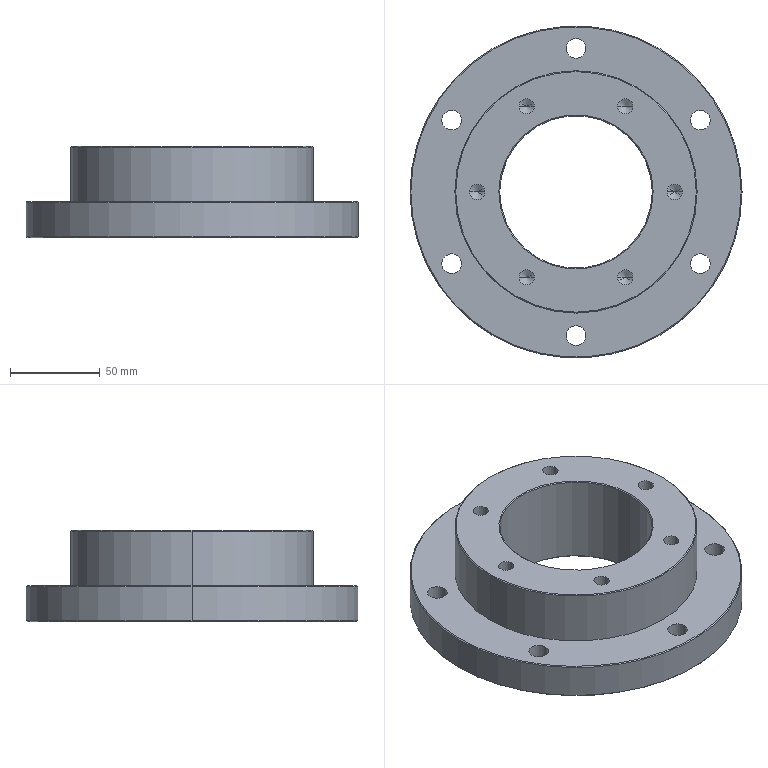Part | SolidWorks | features CirPattern 2, HoleWzd 2, Chamfer 1, Revolution 1 | 1 solid | 73 faces | box 185 x 185 x 51 mm | volume 661113 mm3 | cylinder 42 | cone 22 | plane 9 | commonest cylinder face diameters 8.5 x12 11 x12 18 x12 85 x2 135 x2 185 x2